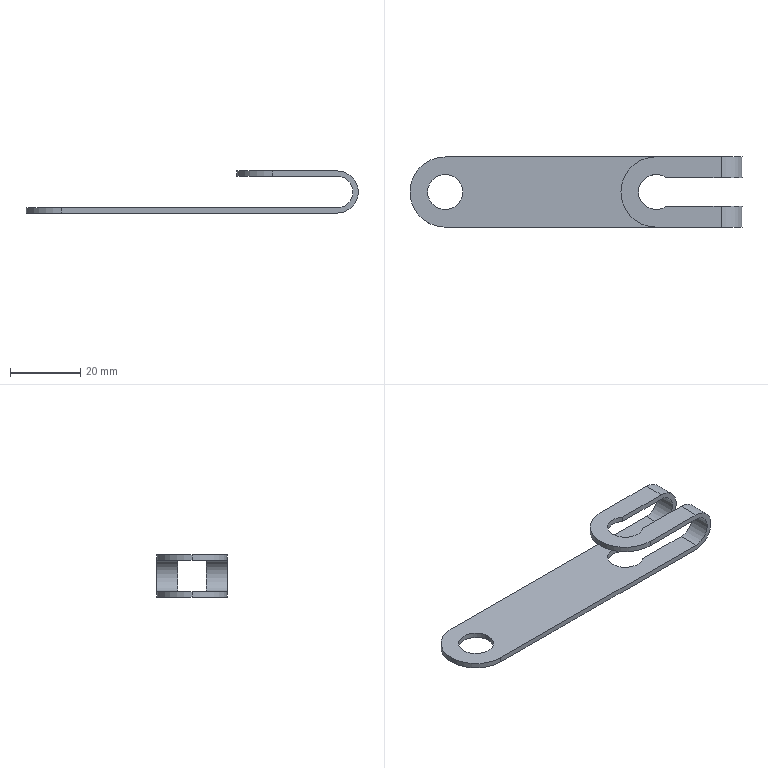Part | SolidWorks | features Extrusion 1, Fillet 1, ICE 1 | 1 solid | 20 faces | box 94.5 x 20 x 12 mm | volume 2986 mm3 | cylinder 12 | plane 8 | commonest cylinder face diameters 10 x4 20 x4 9 x2 12 x2
STEP:
#1=CARTESIAN_POINT('',(-83.5,10.,-6.));
#2=VERTEX_POINT('',#1);
#3=CARTESIAN_POINT('',(-73.5,10.,-6.));
#4=VERTEX_POINT('',#3);
#5=CARTESIAN_POINT('',(-78.5,10.,-6.));
#6=DIRECTION('',(0.,0.,1.));
#7=DIRECTION('',(1.,0.,0.));
#8=AXIS2_PLACEMENT_3D('',#5,#6,#7);
#9=CIRCLE('',#8,5.);
#10=EDGE_CURVE('',#2,#4,#9,.T.);
#11=ORIENTED_EDGE('',*,*,#10,.F.);
#12=CARTESIAN_POINT('',(-83.5,10.,-4.5));
#13=VERTEX_POINT('',#12);
#14=CARTESIAN_POINT('',(-83.5,10.,-6.));
#15=DIRECTION('',(0.,0.,1.));
#16=VECTOR('',#15,1000.);
#17=LINE('',#14,#16);
#18=EDGE_CURVE('',#2,#13,#17,.T.);
#19=ORIENTED_EDGE('',*,*,#18,.T.);
#20=CARTESIAN_POINT('',(-73.5,10.,-4.5));
#21=VERTEX_POINT('',#20);
#22=CARTESIAN_POINT('',(-78.5,10.,-4.5));
#23=DIRECTION('',(0.,0.,-1.));
#24=DIRECTION('',(-1.,0.,0.));
#25=AXIS2_PLACEMENT_3D('',#22,#23,#24);
#26=CIRCLE('',#25,5.);
#27=EDGE_CURVE('',#21,#13,#26,.T.);
#28=ORIENTED_EDGE('',*,*,#27,.F.);
#29=CARTESIAN_POINT('',(-73.5,10.,-6.));
#30=DIRECTION('',(0.,0.,1.));
#31=VECTOR('',#30,1000.);
#32=LINE('',#29,#31);
#33=EDGE_CURVE('',#4,#21,#32,.T.);
#34=ORIENTED_EDGE('',*,*,#33,.F.);
#35=EDGE_LOOP('',(#11,#19,#28,#34));
#36=FACE_OUTER_BOUND('',#35,.T.);
#37=CARTESIAN_POINT('',(-78.5,10.,-6.));
#38=DIRECTION('',(0.,0.,1.));
#39=DIRECTION('',(1.,0.,0.));
#40=AXIS2_PLACEMENT_3D('',#37,#38,#39);
#41=CYLINDRICAL_SURFACE('',#40,5.);
#42=ADVANCED_FACE('',(#36),#41,.F.);
#43=CARTESIAN_POINT('',(0.,20.,6.));
#44=VERTEX_POINT('',#43);
#45=CARTESIAN_POINT('',(0.,14.,6.));
#46=VERTEX_POINT('',#45);
#47=CARTESIAN_POINT('',(0.,20.,6.));
#48=DIRECTION('',(0.,-1.,0.));
#49=VECTOR('',#48,1000.);
#50=LINE('',#47,#49);
#51=EDGE_CURVE('',#44,#46,#50,.T.);
#52=ORIENTED_EDGE('',*,*,#51,.T.);
#53=CARTESIAN_POINT('',(0.,14.,-6.));
#54=VERTEX_POINT('',#53);
#55=CARTESIAN_POINT('',(0.,14.,0.));
#56=DIRECTION('',(0.,1.,0.));
#57=DIRECTION('',(0.,0.,1.));
#58=AXIS2_PLACEMENT_3D('',#55,#56,#57);
#59=CIRCLE('',#58,6.);
#60=EDGE_CURVE('',#46,#54,#59,.T.);
#61=ORIENTED_EDGE('',*,*,#60,.T.);
#62=CARTESIAN_POINT('',(0.,20.,-6.));
#63=VERTEX_POINT('',#62);
#64=CARTESIAN_POINT('',(0.,20.,-6.));
#65=DIRECTION('',(0.,-1.,0.));
#66=VECTOR('',#65,1000.);
#67=LINE('',#64,#66);
#68=EDGE_CURVE('',#63,#54,#67,.T.);
#69=ORIENTED_EDGE('',*,*,#68,.F.);
#70=CARTESIAN_POINT('',(0.,20.,0.));
#71=DIRECTION('',(0.,1.,0.));
#72=DIRECTION('',(0.,0.,1.));
#73=AXIS2_PLACEMENT_3D('',#70,#71,#72);
#74=CIRCLE('',#73,6.);
#75=EDGE_CURVE('',#44,#63,#74,.T.);
#76=ORIENTED_EDGE('',*,*,#75,.F.);
#77=EDGE_LOOP('',(#52,#61,#69,#76));
#78=FACE_OUTER_BOUND('',#77,.T.);
#79=CARTESIAN_POINT('',(0.,20.,0.));
#80=DIRECTION('',(0.,-1.,0.));
#81=DIRECTION('',(0.,0.,-1.));
#82=AXIS2_PLACEMENT_3D('',#79,#80,#81);
#83=CYLINDRICAL_SURFACE('',#82,6.);
#84=ADVANCED_FACE('',(#78),#83,.T.);
#85=CARTESIAN_POINT('',(0.,20.,-4.5));
#86=VERTEX_POINT('',#85);
#87=CARTESIAN_POINT('',(0.,14.,-4.5));
#88=VERTEX_POINT('',#87);
#89=CARTESIAN_POINT('',(0.,20.,-4.5));
#90=DIRECTION('',(0.,-1.,0.));
#91=VECTOR('',#90,1000.);
#92=LINE('',#89,#91);
#93=EDGE_CURVE('',#86,#88,#92,.T.);
#94=ORIENTED_EDGE('',*,*,#93,.T.);
#95=CARTESIAN_POINT('',(0.,14.,4.5));
#96=VERTEX_POINT('',#95);
#97=CARTESIAN_POINT('',(0.,14.,0.));
#98=DIRECTION('',(0.,-1.,0.));
#99=DIRECTION('',(0.,0.,1.));
#100=AXIS2_PLACEMENT_3D('',#97,#98,#99);
#101=CIRCLE('',#100,4.5);
#102=EDGE_CURVE('',#88,#96,#101,.T.);
#103=ORIENTED_EDGE('',*,*,#102,.T.);
#104=CARTESIAN_POINT('',(0.,20.,4.5));
#105=VERTEX_POINT('',#104);
#106=CARTESIAN_POINT('',(0.,20.,4.5));
#107=DIRECTION('',(0.,-1.,0.));
#108=VECTOR('',#107,1000.);
#109=LINE('',#106,#108);
#110=EDGE_CURVE('',#105,#96,#109,.T.);
#111=ORIENTED_EDGE('',*,*,#110,.F.);
#112=CARTESIAN_POINT('',(0.,20.,0.));
#113=DIRECTION('',(0.,-1.,0.));
#114=DIRECTION('',(0.,0.,1.));
#115=AXIS2_PLACEMENT_3D('',#112,#113,#114);
#116=CIRCLE('',#115,4.5);
#117=EDGE_CURVE('',#86,#105,#116,.T.);
#118=ORIENTED_EDGE('',*,*,#117,.F.);
#119=EDGE_LOOP('',(#94,#103,#111,#118));
#120=FACE_OUTER_BOUND('',#119,.T.);
#121=CARTESIAN_POINT('',(0.,20.,0.));
#122=DIRECTION('',(0.,-1.,0.));
#123=DIRECTION('',(0.,0.,-1.));
#124=AXIS2_PLACEMENT_3D('',#121,#122,#123);
#125=CYLINDRICAL_SURFACE('',#124,4.5);
#126=ADVANCED_FACE('',(#120),#125,.F.);
#127=CARTESIAN_POINT('',(0.,6.,-6.));
#128=VERTEX_POINT('',#127);
#129=CARTESIAN_POINT('',(0.,0.,-6.));
#130=VERTEX_POINT('',#129);
#131=CARTESIAN_POINT('',(0.,20.,-6.));
#132=DIRECTION('',(0.,-1.,0.));
#133=VECTOR('',#132,1000.);
#134=LINE('',#131,#133);
#135=EDGE_CURVE('',#128,#130,#134,.T.);
#136=ORIENTED_EDGE('',*,*,#135,.F.);
#137=CARTESIAN_POINT('',(0.,6.,6.));
#138=VERTEX_POINT('',#137);
#139=CARTESIAN_POINT('',(0.,6.,0.));
#140=DIRECTION('',(0.,-1.,0.));
#141=DIRECTION('',(1.,0.,0.));
#142=AXIS2_PLACEMENT_3D('',#139,#140,#141);
#143=CIRCLE('',#142,6.);
#144=EDGE_CURVE('',#128,#138,#143,.T.);
#145=ORIENTED_EDGE('',*,*,#144,.T.);
#146=CARTESIAN_POINT('',(0.,0.,6.));
#147=VERTEX_POINT('',#146);
#148=CARTESIAN_POINT('',(0.,20.,6.));
#149=DIRECTION('',(0.,-1.,0.));
#150=VECTOR('',#149,1000.);
#151=LINE('',#148,#150);
#152=EDGE_CURVE('',#138,#147,#151,.T.);
#153=ORIENTED_EDGE('',*,*,#152,.T.);
#154=CARTESIAN_POINT('',(0.,0.,0.));
#155=DIRECTION('',(0.,1.,0.));
#156=DIRECTION('',(0.,0.,1.));
#157=AXIS2_PLACEMENT_3D('',#154,#155,#156);
#158=CIRCLE('',#157,6.);
#159=EDGE_CURVE('',#147,#130,#158,.T.);
#160=ORIENTED_EDGE('',*,*,#159,.T.);
#161=EDGE_LOOP('',(#136,#145,#153,#160));
#162=FACE_OUTER_BOUND('',#161,.T.);
#163=CARTESIAN_POINT('',(0.,20.,0.));
#164=DIRECTION('',(0.,-1.,0.));
#165=DIRECTION('',(0.,0.,-1.));
#166=AXIS2_PLACEMENT_3D('',#163,#164,#165);
#167=CYLINDRICAL_SURFACE('',#166,6.);
#168=ADVANCED_FACE('',(#162),#167,.T.);
#169=CARTESIAN_POINT('',(-78.5,10.,-6.));
#170=DIRECTION('',(0.,0.,1.));
#171=DIRECTION('',(1.,0.,0.));
#172=AXIS2_PLACEMENT_3D('',#169,#170,#171);
#173=CIRCLE('',#172,5.);
#174=EDGE_CURVE('',#4,#2,#173,.T.);
#175=ORIENTED_EDGE('',*,*,#174,.T.);
#176=ORIENTED_EDGE('',*,*,#10,.T.);
#177=EDGE_LOOP('',(#175,#176));
#178=FACE_BOUND('',#177,.T.);
#179=ORIENTED_EDGE('',*,*,#68,.T.);
#180=CARTESIAN_POINT('',(-15.5,14.,-6.));
#181=VERTEX_POINT('',#180);
#182=CARTESIAN_POINT('',(-15.5,14.,-6.));
#183=DIRECTION('',(-1.,0.,0.));
#184=VECTOR('',#183,1000.);
#185=LINE('',#182,#184);
#186=EDGE_CURVE('',#54,#181,#185,.T.);
#187=ORIENTED_EDGE('',*,*,#186,.T.);
#188=CARTESIAN_POINT('',(-15.5,6.,-6.));
#189=VERTEX_POINT('',#188);
#190=CARTESIAN_POINT('',(-18.5,10.,-6.));
#191=DIRECTION('',(0.,0.,1.));
#192=DIRECTION('',(1.,0.,0.));
#193=AXIS2_PLACEMENT_3D('',#190,#191,#192);
#194=CIRCLE('',#193,5.);
#195=EDGE_CURVE('',#181,#189,#194,.T.);
#196=ORIENTED_EDGE('',*,*,#195,.T.);
#197=CARTESIAN_POINT('',(-15.5,6.,-6.));
#198=DIRECTION('',(1.,0.,0.));
#199=VECTOR('',#198,1000.);
#200=LINE('',#197,#199);
#201=EDGE_CURVE('',#189,#128,#200,.T.);
#202=ORIENTED_EDGE('',*,*,#201,.T.);
#203=ORIENTED_EDGE('',*,*,#135,.T.);
#204=CARTESIAN_POINT('',(-78.5,0.,-6.));
#205=VERTEX_POINT('',#204);
#206=CARTESIAN_POINT('',(0.,0.,-6.));
#207=DIRECTION('',(-1.,0.,0.));
#208=VECTOR('',#207,1000.);
#209=LINE('',#206,#208);
#210=EDGE_CURVE('',#130,#205,#209,.T.);
#211=ORIENTED_EDGE('',*,*,#210,.T.);
#212=CARTESIAN_POINT('',(-88.5,10.,-6.));
#213=VERTEX_POINT('',#212);
#214=CARTESIAN_POINT('',(-78.5,10.,-6.));
#215=DIRECTION('',(0.,0.,-1.));
#216=DIRECTION('',(1.,0.,0.));
#217=AXIS2_PLACEMENT_3D('',#214,#215,#216);
#218=CIRCLE('',#217,10.);
#219=EDGE_CURVE('',#205,#213,#218,.T.);
#220=ORIENTED_EDGE('',*,*,#219,.T.);
#221=CARTESIAN_POINT('',(-78.5,20.,-6.));
#222=VERTEX_POINT('',#221);
#223=CARTESIAN_POINT('',(-78.5,10.,-6.));
#224=DIRECTION('',(0.,0.,-1.));
#225=DIRECTION('',(1.,0.,0.));
#226=AXIS2_PLACEMENT_3D('',#223,#224,#225);
#227=CIRCLE('',#226,10.);
#228=EDGE_CURVE('',#213,#222,#227,.T.);
#229=ORIENTED_EDGE('',*,*,#228,.T.);
#230=CARTESIAN_POINT('',(0.,20.,-6.));
#231=DIRECTION('',(-1.,0.,0.));
#232=VECTOR('',#231,1000.);
#233=LINE('',#230,#232);
#234=EDGE_CURVE('',#63,#222,#233,.T.);
#235=ORIENTED_EDGE('',*,*,#234,.F.);
#236=EDGE_LOOP('',(#179,#187,#196,#202,#203,#211,#220,#229,#235));
#237=FACE_OUTER_BOUND('',#236,.T.);
#238=CARTESIAN_POINT('',(0.,20.,-6.));
#239=DIRECTION('',(0.,0.,1.));
#240=DIRECTION('',(1.,0.,0.));
#241=AXIS2_PLACEMENT_3D('',#238,#239,#240);
#242=PLANE('',#241);
#243=ADVANCED_FACE('',(#178,#237),#242,.F.);
#244=ORIENTED_EDGE('',*,*,#27,.T.);
#245=CARTESIAN_POINT('',(-78.5,10.,-4.5));
#246=DIRECTION('',(0.,0.,-1.));
#247=DIRECTION('',(-1.,0.,0.));
#248=AXIS2_PLACEMENT_3D('',#245,#246,#247);
#249=CIRCLE('',#248,5.);
#250=EDGE_CURVE('',#13,#21,#249,.T.);
#251=ORIENTED_EDGE('',*,*,#250,.T.);
#252=EDGE_LOOP('',(#244,#251));
#253=FACE_BOUND('',#252,.T.);
#254=CARTESIAN_POINT('',(-15.5,6.,-4.5));
#255=VERTEX_POINT('',#254);
#256=CARTESIAN_POINT('',(-15.5,14.,-4.5));
#257=VERTEX_POINT('',#256);
#258=CARTESIAN_POINT('',(-18.5,10.,-4.5));
#259=DIRECTION('',(0.,0.,-1.));
#260=DIRECTION('',(-1.,0.,0.));
#261=AXIS2_PLACEMENT_3D('',#258,#259,#260);
#262=CIRCLE('',#261,5.);
#263=EDGE_CURVE('',#255,#257,#262,.T.);
#264=ORIENTED_EDGE('',*,*,#263,.T.);
#265=CARTESIAN_POINT('',(-88.5,14.,-4.5));
#266=DIRECTION('',(1.,0.,0.));
#267=VECTOR('',#266,1000.);
#268=LINE('',#265,#267);
#269=EDGE_CURVE('',#257,#88,#268,.T.);
#270=ORIENTED_EDGE('',*,*,#269,.T.);
#271=ORIENTED_EDGE('',*,*,#93,.F.);
#272=CARTESIAN_POINT('',(-78.5,20.,-4.5));
#273=VERTEX_POINT('',#272);
#274=CARTESIAN_POINT('',(-88.5,20.,-4.5));
#275=DIRECTION('',(1.,0.,0.));
#276=VECTOR('',#275,1000.);
#277=LINE('',#274,#276);
#278=EDGE_CURVE('',#273,#86,#277,.T.);
#279=ORIENTED_EDGE('',*,*,#278,.F.);
#280=CARTESIAN_POINT('',(-88.5,10.,-4.5));
#281=VERTEX_POINT('',#280);
#282=CARTESIAN_POINT('',(-78.5,10.,-4.5));
#283=DIRECTION('',(0.,0.,1.));
#284=DIRECTION('',(-1.,0.,0.));
#285=AXIS2_PLACEMENT_3D('',#282,#283,#284);
#286=CIRCLE('',#285,10.);
#287=EDGE_CURVE('',#273,#281,#286,.T.);
#288=ORIENTED_EDGE('',*,*,#287,.T.);
#289=CARTESIAN_POINT('',(-78.5,0.,-4.5));
#290=VERTEX_POINT('',#289);
#291=CARTESIAN_POINT('',(-78.5,10.,-4.5));
#292=DIRECTION('',(0.,0.,1.));
#293=DIRECTION('',(-1.,0.,0.));
#294=AXIS2_PLACEMENT_3D('',#291,#292,#293);
#295=CIRCLE('',#294,10.);
#296=EDGE_CURVE('',#281,#290,#295,.T.);
#297=ORIENTED_EDGE('',*,*,#296,.T.);
#298=CARTESIAN_POINT('',(0.,0.,-4.5));
#299=VERTEX_POINT('',#298);
#300=CARTESIAN_POINT('',(-88.5,0.,-4.5));
#301=DIRECTION('',(1.,0.,0.));
#302=VECTOR('',#301,1000.);
#303=LINE('',#300,#302);
#304=EDGE_CURVE('',#290,#299,#303,.T.);
#305=ORIENTED_EDGE('',*,*,#304,.T.);
#306=CARTESIAN_POINT('',(0.,6.,-4.5));
#307=VERTEX_POINT('',#306);
#308=CARTESIAN_POINT('',(0.,20.,-4.5));
#309=DIRECTION('',(0.,-1.,0.));
#310=VECTOR('',#309,1000.);
#311=LINE('',#308,#310);
#312=EDGE_CURVE('',#307,#299,#311,.T.);
#313=ORIENTED_EDGE('',*,*,#312,.F.);
#314=CARTESIAN_POINT('',(-88.5,6.,-4.5));
#315=DIRECTION('',(-1.,0.,0.));
#316=VECTOR('',#315,1000.);
#317=LINE('',#314,#316);
#318=EDGE_CURVE('',#307,#255,#317,.T.);
#319=ORIENTED_EDGE('',*,*,#318,.T.);
#320=EDGE_LOOP('',(#264,#270,#271,#279,#288,#297,#305,#313,#319));
#321=FACE_OUTER_BOUND('',#320,.T.);
#322=CARTESIAN_POINT('',(-88.5,20.,-4.5));
#323=DIRECTION('',(0.,0.,-1.));
#324=DIRECTION('',(-1.,0.,0.));
#325=AXIS2_PLACEMENT_3D('',#322,#323,#324);
#326=PLANE('',#325);
#327=ADVANCED_FACE('',(#253,#321),#326,.F.);
#328=CARTESIAN_POINT('',(0.,6.,4.5));
#329=VERTEX_POINT('',#328);
#330=CARTESIAN_POINT('',(0.,0.,4.5));
#331=VERTEX_POINT('',#330);
#332=CARTESIAN_POINT('',(0.,20.,4.5));
#333=DIRECTION('',(0.,-1.,0.));
#334=VECTOR('',#333,1000.);
#335=LINE('',#332,#334);
#336=EDGE_CURVE('',#329,#331,#335,.T.);
#337=ORIENTED_EDGE('',*,*,#336,.F.);
#338=CARTESIAN_POINT('',(0.,6.,0.));
#339=DIRECTION('',(0.,1.,0.));
#340=DIRECTION('',(1.,0.,0.));
#341=AXIS2_PLACEMENT_3D('',#338,#339,#340);
#342=CIRCLE('',#341,4.5);
#343=EDGE_CURVE('',#329,#307,#342,.T.);
#344=ORIENTED_EDGE('',*,*,#343,.T.);
#345=ORIENTED_EDGE('',*,*,#312,.T.);
#346=CARTESIAN_POINT('',(0.,0.,0.));
#347=DIRECTION('',(0.,-1.,0.));
#348=DIRECTION('',(0.,0.,1.));
#349=AXIS2_PLACEMENT_3D('',#346,#347,#348);
#350=CIRCLE('',#349,4.5);
#351=EDGE_CURVE('',#299,#331,#350,.T.);
#352=ORIENTED_EDGE('',*,*,#351,.T.);
#353=EDGE_LOOP('',(#337,#344,#345,#352));
#354=FACE_OUTER_BOUND('',#353,.T.);
#355=CARTESIAN_POINT('',(0.,20.,0.));
#356=DIRECTION('',(0.,-1.,0.));
#357=DIRECTION('',(0.,0.,-1.));
#358=AXIS2_PLACEMENT_3D('',#355,#356,#357);
#359=CYLINDRICAL_SURFACE('',#358,4.5);
#360=ADVANCED_FACE('',(#354),#359,.F.);
#361=ORIENTED_EDGE('',*,*,#110,.T.);
#362=CARTESIAN_POINT('',(-15.5,14.,4.5));
#363=VERTEX_POINT('',#362);
#364=CARTESIAN_POINT('',(-28.5,14.,4.5));
#365=DIRECTION('',(-1.,0.,0.));
#366=VECTOR('',#365,1000.);
#367=LINE('',#364,#366);
#368=EDGE_CURVE('',#96,#363,#367,.T.);
#369=ORIENTED_EDGE('',*,*,#368,.T.);
#370=CARTESIAN_POINT('',(-15.5,6.,4.5));
#371=VERTEX_POINT('',#370);
#372=CARTESIAN_POINT('',(-18.5,10.,4.5));
#373=DIRECTION('',(0.,0.,1.));
#374=DIRECTION('',(1.,0.,0.));
#375=AXIS2_PLACEMENT_3D('',#372,#373,#374);
#376=CIRCLE('',#375,5.);
#377=EDGE_CURVE('',#363,#371,#376,.T.);
#378=ORIENTED_EDGE('',*,*,#377,.T.);
#379=CARTESIAN_POINT('',(-28.5,6.,4.5));
#380=DIRECTION('',(1.,0.,0.));
#381=VECTOR('',#380,1000.);
#382=LINE('',#379,#381);
#383=EDGE_CURVE('',#371,#329,#382,.T.);
#384=ORIENTED_EDGE('',*,*,#383,.T.);
#385=ORIENTED_EDGE('',*,*,#336,.T.);
#386=CARTESIAN_POINT('',(-18.5,0.,4.5));
#387=VERTEX_POINT('',#386);
#388=CARTESIAN_POINT('',(-28.5,0.,4.5));
#389=DIRECTION('',(-1.,0.,0.));
#390=VECTOR('',#389,1000.);
#391=LINE('',#388,#390);
#392=EDGE_CURVE('',#331,#387,#391,.T.);
#393=ORIENTED_EDGE('',*,*,#392,.T.);
#394=CARTESIAN_POINT('',(-28.5,10.,4.5));
#395=VERTEX_POINT('',#394);
#396=CARTESIAN_POINT('',(-18.5,10.,4.5));
#397=DIRECTION('',(0.,0.,-1.));
#398=DIRECTION('',(1.,0.,0.));
#399=AXIS2_PLACEMENT_3D('',#396,#397,#398);
#400=CIRCLE('',#399,10.);
#401=EDGE_CURVE('',#387,#395,#400,.T.);
#402=ORIENTED_EDGE('',*,*,#401,.T.);
#403=CARTESIAN_POINT('',(-18.5,20.,4.5));
#404=VERTEX_POINT('',#403);
#405=CARTESIAN_POINT('',(-18.5,10.,4.5));
#406=DIRECTION('',(0.,0.,-1.));
#407=DIRECTION('',(1.,0.,0.));
#408=AXIS2_PLACEMENT_3D('',#405,#406,#407);
#409=CIRCLE('',#408,10.);
#410=EDGE_CURVE('',#395,#404,#409,.T.);
#411=ORIENTED_EDGE('',*,*,#410,.T.);
#412=CARTESIAN_POINT('',(-28.5,20.,4.5));
#413=DIRECTION('',(-1.,0.,0.));
#414=VECTOR('',#413,1000.);
#415=LINE('',#412,#414);
#416=EDGE_CURVE('',#105,#404,#415,.T.);
#417=ORIENTED_EDGE('',*,*,#416,.F.);
#418=EDGE_LOOP('',(#361,#369,#378,#384,#385,#393,#402,#411,#417));
#419=FACE_OUTER_BOUND('',#418,.T.);
#420=CARTESIAN_POINT('',(-28.5,20.,4.5));
#421=DIRECTION('',(0.,0.,1.));
#422=DIRECTION('',(1.,0.,0.));
#423=AXIS2_PLACEMENT_3D('',#420,#421,#422);
#424=PLANE('',#423);
#425=ADVANCED_FACE('',(#419),#424,.F.);
#426=CARTESIAN_POINT('',(-15.5,14.,6.));
#427=VERTEX_POINT('',#426);
#428=CARTESIAN_POINT('',(-15.5,6.,6.));
#429=VERTEX_POINT('',#428);
#430=CARTESIAN_POINT('',(-18.5,10.,6.));
#431=DIRECTION('',(0.,0.,1.));
#432=DIRECTION('',(1.,0.,0.));
#433=AXIS2_PLACEMENT_3D('',#430,#431,#432);
#434=CIRCLE('',#433,5.);
#435=EDGE_CURVE('',#427,#429,#434,.T.);
#436=ORIENTED_EDGE('',*,*,#435,.F.);
#437=CARTESIAN_POINT('',(0.,14.,6.));
#438=DIRECTION('',(1.,0.,0.));
#439=VECTOR('',#438,1000.);
#440=LINE('',#437,#439);
#441=EDGE_CURVE('',#427,#46,#440,.T.);
#442=ORIENTED_EDGE('',*,*,#441,.T.);
#443=ORIENTED_EDGE('',*,*,#51,.F.);
#444=CARTESIAN_POINT('',(-18.5,20.,6.));
#445=VERTEX_POINT('',#444);
#446=CARTESIAN_POINT('',(0.,20.,6.));
#447=DIRECTION('',(1.,0.,0.));
#448=VECTOR('',#447,1000.);
#449=LINE('',#446,#448);
#450=EDGE_CURVE('',#445,#44,#449,.T.);
#451=ORIENTED_EDGE('',*,*,#450,.F.);
#452=CARTESIAN_POINT('',(-28.5,10.,6.));
#453=VERTEX_POINT('',#452);
#454=CARTESIAN_POINT('',(-18.5,10.,6.));
#455=DIRECTION('',(0.,0.,1.));
#456=DIRECTION('',(-1.,0.,0.));
#457=AXIS2_PLACEMENT_3D('',#454,#455,#456);
#458=CIRCLE('',#457,10.);
#459=EDGE_CURVE('',#445,#453,#458,.T.);
#460=ORIENTED_EDGE('',*,*,#459,.T.);
#461=CARTESIAN_POINT('',(-18.5,0.,6.));
#462=VERTEX_POINT('',#461);
#463=CARTESIAN_POINT('',(-18.5,10.,6.));
#464=DIRECTION('',(0.,0.,1.));
#465=DIRECTION('',(-1.,0.,0.));
#466=AXIS2_PLACEMENT_3D('',#463,#464,#465);
#467=CIRCLE('',#466,10.);
#468=EDGE_CURVE('',#453,#462,#467,.T.);
#469=ORIENTED_EDGE('',*,*,#468,.T.);
#470=CARTESIAN_POINT('',(0.,0.,6.));
#471=DIRECTION('',(1.,0.,0.));
#472=VECTOR('',#471,1000.);
#473=LINE('',#470,#472);
#474=EDGE_CURVE('',#462,#147,#473,.T.);
#475=ORIENTED_EDGE('',*,*,#474,.T.);
#476=ORIENTED_EDGE('',*,*,#152,.F.);
#477=CARTESIAN_POINT('',(-15.5,6.,6.));
#478=DIRECTION('',(1.,0.,0.));
#479=VECTOR('',#478,1000.);
#480=LINE('',#477,#479);
#481=EDGE_CURVE('',#429,#138,#480,.T.);
#482=ORIENTED_EDGE('',*,*,#481,.F.);
#483=EDGE_LOOP('',(#436,#442,#443,#451,#460,#469,#475,#476,#482));
#484=FACE_OUTER_BOUND('',#483,.T.);
#485=CARTESIAN_POINT('',(0.,20.,6.));
#486=DIRECTION('',(0.,0.,-1.));
#487=DIRECTION('',(-1.,0.,0.));
#488=AXIS2_PLACEMENT_3D('',#485,#486,#487);
#489=PLANE('',#488);
#490=ADVANCED_FACE('',(#484),#489,.F.);
#491=ORIENTED_EDGE('',*,*,#416,.T.);
#492=CARTESIAN_POINT('',(-18.5,20.,6.));
#493=DIRECTION('',(0.,0.,1.));
#494=VECTOR('',#493,1000.);
#495=LINE('',#492,#494);
#496=EDGE_CURVE('',#404,#445,#495,.T.);
#497=ORIENTED_EDGE('',*,*,#496,.T.);
#498=ORIENTED_EDGE('',*,*,#450,.T.);
#499=ORIENTED_EDGE('',*,*,#75,.T.);
#500=ORIENTED_EDGE('',*,*,#234,.T.);
#501=CARTESIAN_POINT('',(-78.5,20.,-4.5));
#502=DIRECTION('',(0.,0.,1.));
#503=VECTOR('',#502,1000.);
#504=LINE('',#501,#503);
#505=EDGE_CURVE('',#222,#273,#504,.T.);
#506=ORIENTED_EDGE('',*,*,#505,.T.);
#507=ORIENTED_EDGE('',*,*,#278,.T.);
#508=ORIENTED_EDGE('',*,*,#117,.T.);
#509=EDGE_LOOP('',(#491,#497,#498,#499,#500,#506,#507,#508));
#510=FACE_OUTER_BOUND('',#509,.T.);
#511=CARTESIAN_POINT('',(0.,20.,0.));
#512=DIRECTION('',(0.,1.,0.));
#513=DIRECTION('',(0.,0.,1.));
#514=AXIS2_PLACEMENT_3D('',#511,#512,#513);
#515=PLANE('',#514);
#516=ADVANCED_FACE('',(#510),#515,.T.);
#517=ORIENTED_EDGE('',*,*,#474,.F.);
#518=CARTESIAN_POINT('',(-18.5,0.,0.));
#519=DIRECTION('',(0.,0.,-1.));
#520=VECTOR('',#519,1000.);
#521=LINE('',#518,#520);
#522=EDGE_CURVE('',#462,#387,#521,.T.);
#523=ORIENTED_EDGE('',*,*,#522,.T.);
#524=ORIENTED_EDGE('',*,*,#392,.F.);
#525=ORIENTED_EDGE('',*,*,#351,.F.);
#526=ORIENTED_EDGE('',*,*,#304,.F.);
#527=CARTESIAN_POINT('',(-78.5,0.,0.));
#528=DIRECTION('',(0.,0.,-1.));
#529=VECTOR('',#528,1000.);
#530=LINE('',#527,#529);
#531=EDGE_CURVE('',#290,#205,#530,.T.);
#532=ORIENTED_EDGE('',*,*,#531,.T.);
#533=ORIENTED_EDGE('',*,*,#210,.F.);
#534=ORIENTED_EDGE('',*,*,#159,.F.);
#535=EDGE_LOOP('',(#517,#523,#524,#525,#526,#532,#533,#534));
#536=FACE_OUTER_BOUND('',#535,.T.);
#537=CARTESIAN_POINT('',(0.,0.,0.));
#538=DIRECTION('',(0.,1.,0.));
#539=DIRECTION('',(0.,0.,1.));
#540=AXIS2_PLACEMENT_3D('',#537,#538,#539);
#541=PLANE('',#540);
#542=ADVANCED_FACE('',(#536),#541,.F.);
#543=ORIENTED_EDGE('',*,*,#496,.F.);
#544=ORIENTED_EDGE('',*,*,#410,.F.);
#545=CARTESIAN_POINT('',(-28.5,10.,4.5));
#546=DIRECTION('',(0.,0.,-1.));
#547=VECTOR('',#546,1000.);
#548=LINE('',#545,#547);
#549=EDGE_CURVE('',#453,#395,#548,.T.);
#550=ORIENTED_EDGE('',*,*,#549,.F.);
#551=ORIENTED_EDGE('',*,*,#459,.F.);
#552=EDGE_LOOP('',(#543,#544,#550,#551));
#553=FACE_OUTER_BOUND('',#552,.T.);
#554=CARTESIAN_POINT('',(-18.5,10.,0.));
#555=DIRECTION('',(0.,0.,-1.));
#556=DIRECTION('',(-1.,0.,0.));
#557=AXIS2_PLACEMENT_3D('',#554,#555,#556);
#558=CYLINDRICAL_SURFACE('',#557,10.);
#559=ADVANCED_FACE('',(#553),#558,.T.);
#560=ORIENTED_EDGE('',*,*,#401,.F.);
#561=ORIENTED_EDGE('',*,*,#522,.F.);
#562=ORIENTED_EDGE('',*,*,#468,.F.);
#563=ORIENTED_EDGE('',*,*,#549,.T.);
#564=EDGE_LOOP('',(#560,#561,#562,#563));
#565=FACE_OUTER_BOUND('',#564,.T.);
#566=CARTESIAN_POINT('',(-18.5,10.,6.));
#567=DIRECTION('',(0.,0.,1.));
#568=DIRECTION('',(1.,0.,0.));
#569=AXIS2_PLACEMENT_3D('',#566,#567,#568);
#570=CYLINDRICAL_SURFACE('',#569,10.);
#571=ADVANCED_FACE('',(#565),#570,.T.);
#572=ORIENTED_EDGE('',*,*,#505,.F.);
#573=ORIENTED_EDGE('',*,*,#228,.F.);
#574=CARTESIAN_POINT('',(-88.5,10.,-6.));
#575=DIRECTION('',(0.,0.,-1.));
#576=VECTOR('',#575,1000.);
#577=LINE('',#574,#576);
#578=EDGE_CURVE('',#281,#213,#577,.T.);
#579=ORIENTED_EDGE('',*,*,#578,.F.);
#580=ORIENTED_EDGE('',*,*,#287,.F.);
#581=EDGE_LOOP('',(#572,#573,#579,#580));
#582=FACE_OUTER_BOUND('',#581,.T.);
#583=CARTESIAN_POINT('',(-78.5,10.,0.));
#584=DIRECTION('',(0.,0.,-1.));
#585=DIRECTION('',(-1.,0.,0.));
#586=AXIS2_PLACEMENT_3D('',#583,#584,#585);
#587=CYLINDRICAL_SURFACE('',#586,10.);
#588=ADVANCED_FACE('',(#582),#587,.T.);
#589=ORIENTED_EDGE('',*,*,#219,.F.);
#590=ORIENTED_EDGE('',*,*,#531,.F.);
#591=ORIENTED_EDGE('',*,*,#296,.F.);
#592=ORIENTED_EDGE('',*,*,#578,.T.);
#593=EDGE_LOOP('',(#589,#590,#591,#592));
#594=FACE_OUTER_BOUND('',#593,.T.);
#595=CARTESIAN_POINT('',(-78.5,10.,-6.));
#596=DIRECTION('',(0.,0.,1.));
#597=DIRECTION('',(1.,0.,0.));
#598=AXIS2_PLACEMENT_3D('',#595,#596,#597);
#599=CYLINDRICAL_SURFACE('',#598,10.);
#600=ADVANCED_FACE('',(#594),#599,.T.);
#601=CARTESIAN_POINT('',(-15.5,6.,-6.));
#602=DIRECTION('',(0.,0.,1.));
#603=VECTOR('',#602,1000.);
#604=LINE('',#601,#603);
#605=EDGE_CURVE('',#189,#255,#604,.T.);
#606=ORIENTED_EDGE('',*,*,#605,.F.);
#607=ORIENTED_EDGE('',*,*,#195,.F.);
#608=CARTESIAN_POINT('',(-15.5,14.,-6.));
#609=DIRECTION('',(0.,0.,1.));
#610=VECTOR('',#609,1000.);
#611=LINE('',#608,#610);
#612=EDGE_CURVE('',#181,#257,#611,.T.);
#613=ORIENTED_EDGE('',*,*,#612,.T.);
#614=ORIENTED_EDGE('',*,*,#263,.F.);
#615=EDGE_LOOP('',(#606,#607,#613,#614));
#616=FACE_OUTER_BOUND('',#615,.T.);
#617=CARTESIAN_POINT('',(-18.5,10.,-6.));
#618=DIRECTION('',(0.,0.,1.));
#619=DIRECTION('',(1.,0.,0.));
#620=AXIS2_PLACEMENT_3D('',#617,#618,#619);
#621=CYLINDRICAL_SURFACE('',#620,5.);
#622=ADVANCED_FACE('',(#616),#621,.F.);
#623=CARTESIAN_POINT('',(-15.5,14.,-6.));
#624=DIRECTION('',(0.,0.,1.));
#625=VECTOR('',#624,1000.);
#626=LINE('',#623,#625);
#627=EDGE_CURVE('',#363,#427,#626,.T.);
#628=ORIENTED_EDGE('',*,*,#627,.T.);
#629=ORIENTED_EDGE('',*,*,#435,.T.);
#630=CARTESIAN_POINT('',(-15.5,6.,-6.));
#631=DIRECTION('',(0.,0.,1.));
#632=VECTOR('',#631,1000.);
#633=LINE('',#630,#632);
#634=EDGE_CURVE('',#371,#429,#633,.T.);
#635=ORIENTED_EDGE('',*,*,#634,.F.);
#636=ORIENTED_EDGE('',*,*,#377,.F.);
#637=EDGE_LOOP('',(#628,#629,#635,#636));
#638=FACE_OUTER_BOUND('',#637,.T.);
#639=CARTESIAN_POINT('',(-18.5,10.,-6.));
#640=DIRECTION('',(0.,0.,1.));
#641=DIRECTION('',(1.,0.,0.));
#642=AXIS2_PLACEMENT_3D('',#639,#640,#641);
#643=CYLINDRICAL_SURFACE('',#642,5.);
#644=ADVANCED_FACE('',(#638),#643,.F.);
#645=ORIENTED_EDGE('',*,*,#441,.F.);
#646=ORIENTED_EDGE('',*,*,#627,.F.);
#647=ORIENTED_EDGE('',*,*,#368,.F.);
#648=ORIENTED_EDGE('',*,*,#102,.F.);
#649=ORIENTED_EDGE('',*,*,#269,.F.);
#650=ORIENTED_EDGE('',*,*,#612,.F.);
#651=ORIENTED_EDGE('',*,*,#186,.F.);
#652=ORIENTED_EDGE('',*,*,#60,.F.);
#653=EDGE_LOOP('',(#645,#646,#647,#648,#649,#650,#651,#652));
#654=FACE_OUTER_BOUND('',#653,.T.);
#655=CARTESIAN_POINT('',(-15.5,14.,-6.));
#656=DIRECTION('',(0.,1.,0.));
#657=DIRECTION('',(0.,0.,1.));
#658=AXIS2_PLACEMENT_3D('',#655,#656,#657);
#659=PLANE('',#658);
#660=ADVANCED_FACE('',(#654),#659,.F.);
#661=ORIENTED_EDGE('',*,*,#201,.F.);
#662=ORIENTED_EDGE('',*,*,#605,.T.);
#663=ORIENTED_EDGE('',*,*,#318,.F.);
#664=ORIENTED_EDGE('',*,*,#343,.F.);
#665=ORIENTED_EDGE('',*,*,#383,.F.);
#666=ORIENTED_EDGE('',*,*,#634,.T.);
#667=ORIENTED_EDGE('',*,*,#481,.T.);
#668=ORIENTED_EDGE('',*,*,#144,.F.);
#669=EDGE_LOOP('',(#661,#662,#663,#664,#665,#666,#667,#668));
#670=FACE_OUTER_BOUND('',#669,.T.);
#671=CARTESIAN_POINT('',(-15.5,6.,-6.));
#672=DIRECTION('',(0.,-1.,0.));
#673=DIRECTION('',(1.,0.,0.));
#674=AXIS2_PLACEMENT_3D('',#671,#672,#673);
#675=PLANE('',#674);
#676=ADVANCED_FACE('',(#670),#675,.F.);
#677=ORIENTED_EDGE('',*,*,#18,.F.);
#678=ORIENTED_EDGE('',*,*,#174,.F.);
#679=ORIENTED_EDGE('',*,*,#33,.T.);
#680=ORIENTED_EDGE('',*,*,#250,.F.);
#681=EDGE_LOOP('',(#677,#678,#679,#680));
#682=FACE_OUTER_BOUND('',#681,.T.);
#683=CARTESIAN_POINT('',(-78.5,10.,-6.));
#684=DIRECTION('',(0.,0.,1.));
#685=DIRECTION('',(1.,0.,0.));
#686=AXIS2_PLACEMENT_3D('',#683,#684,#685);
#687=CYLINDRICAL_SURFACE('',#686,5.);
#688=ADVANCED_FACE('',(#682),#687,.F.);
#689=CLOSED_SHELL('',(#42,#84,#126,#168,#243,#327,#360,#425,#490,#516,#542,#559,#571,#588,#600,#622,#644,#660,#676,#688));
#690=MANIFOLD_SOLID_BREP('',#689);
#691=CARTESIAN_POINT('',(0.,0.,0.));
#692=DIRECTION('',(0.,0.,1.));
#693=DIRECTION('',(1.,0.,0.));
#694=AXIS2_PLACEMENT_3D('',#691,#692,#693);
#695=(LENGTH_UNIT()NAMED_UNIT(*)SI_UNIT(.MILLI.,.METRE.));
#696=UNCERTAINTY_MEASURE_WITH_UNIT(LENGTH_MEASURE(0.00001),#695,'','');
#697=(NAMED_UNIT(*)PLANE_ANGLE_UNIT()SI_UNIT($,.RADIAN.));
#698=(NAMED_UNIT(*)SI_UNIT($,.STERADIAN.)SOLID_ANGLE_UNIT());
#699=(GEOMETRIC_REPRESENTATION_CONTEXT(3)GLOBAL_UNCERTAINTY_ASSIGNED_CONTEXT((#696))GLOBAL_UNIT_ASSIGNED_CONTEXT((#695,#697,#698))REPRESENTATION_CONTEXT('',''));
#700=ADVANCED_BREP_SHAPE_REPRESENTATION('',(#690,#694),#699);